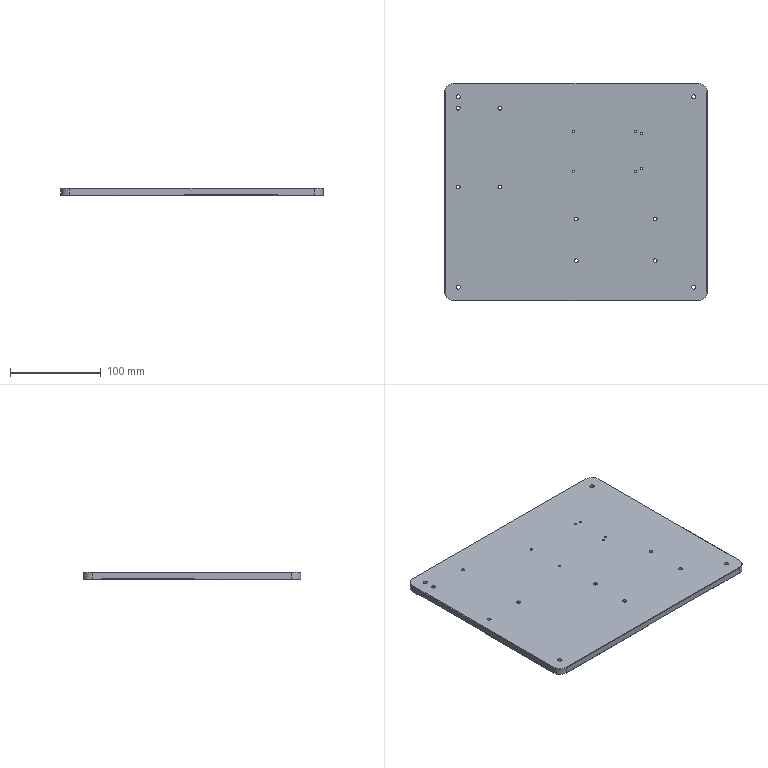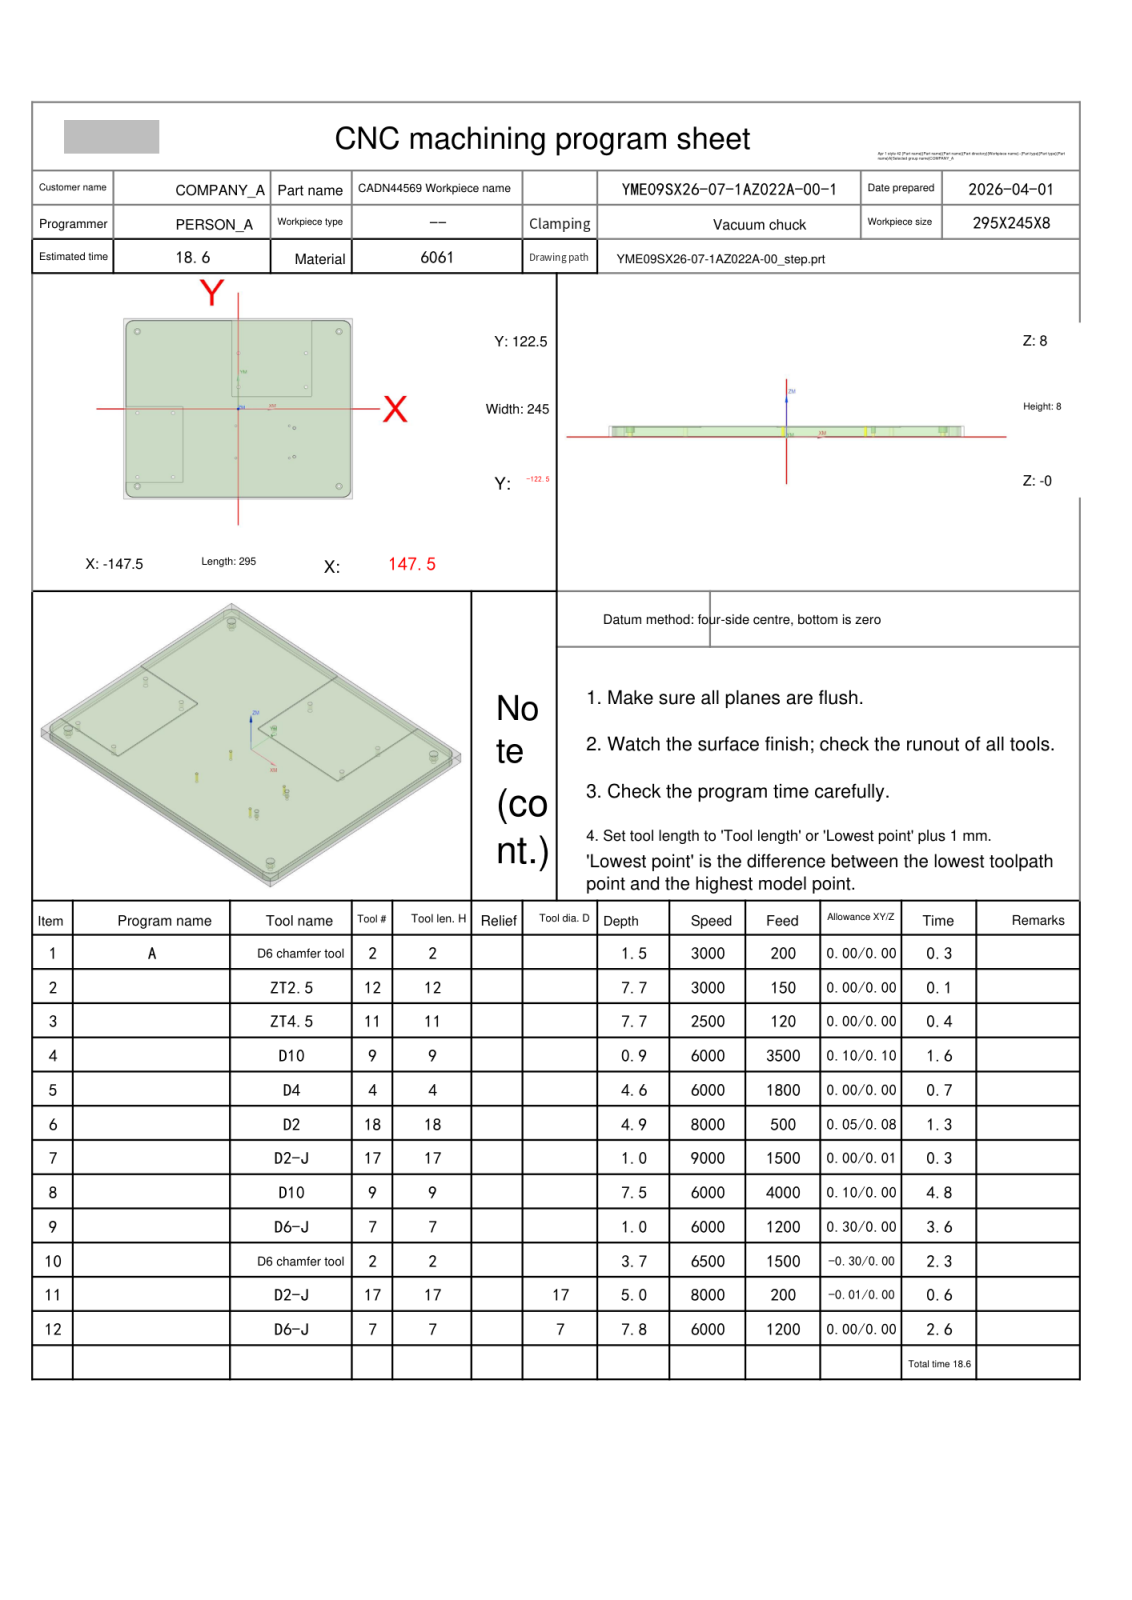NC program | NX | posted by the shop | part box 290 x 240 x 8 mm
Lines 2079 to 2318 of 2318:
N11 T17 M06
(D2-J  D=2. R=0. H=17 ce=-0.01 di=0.00)
G00 G90 G54 X71.195 Y-25.851 M03 S8000
G43 H17 Z28.
M08
Z8.5
G01 Y-25.991 Z8.493 F200.
X71.26 Y-26.261 Z8.478
X71.396 Y-26.503 Z8.464
X71.592 Y-26.699 Z8.449
X71.834 Y-26.835 Z8.434
X72.104 Y-26.9 Z8.42
X72.305 Z8.409
X72.568 Y-26.838 Z8.395
X72.806 Y-26.708 Z8.381
X73. Y-26.521 Z8.367
X73.138 Y-26.288 Z8.353
X73.21 Y-26.027 Z8.339
X73.215 Y-25.79 Z8.326
X73.15 Y-25.52 Z8.312
X73.014 Y-25.278 Z8.297
X72.817 Y-25.081 Z8.282
X72.575 Y-24.945 Z8.268
X72.305 Y-24.88 Z8.253
X72.104 Z8.243
X71.834 Y-24.945 Z8.228
X71.592 Y-25.081 Z8.214
X71.396 Y-25.278 Z8.199
X71.26 Y-25.52 Z8.185
X71.195 Y-25.79 Z8.17
Y-25.991 Z8.159
X71.26 Y-26.261 Z8.145
X71.396 Y-26.503 Z8.13
X71.592 Y-26.699 Z8.116
X71.834 Y-26.835 Z8.101
X72.104 Y-26.9 Z8.087
X72.305 Z8.076
X72.568 Y-26.838 Z8.062
X72.806 Y-26.708 Z8.048
X73. Y-26.521 Z8.034
X73.138 Y-26.288 Z8.019
X73.21 Y-26.027 Z8.005
X73.214 Y-25.927 Z8.
X73.179 Y-25.926
G41 D17
X73.215 Y-25.89
G03 X72.205 Y-24.88 Z7.792 I-1.01 J0.0
X71.195 Y-25.89 Z7.583 I0.0 J-1.01
X72.205 Y-26.9 Z7.375 I1.01 J0.0
X73.215 Y-25.89 Z7.167 I0.0 J1.01
X72.205 Y-24.88 Z6.958 I-1.01 J0.0
X71.195 Y-25.89 Z6.75 I0.0 J-1.01
X72.205 Y-26.9 Z6.542 I1.01 J0.0
X73.215 Y-25.89 Z6.333 I0.0 J1.01
X72.205 Y-24.88 Z6.125 I-1.01 J0.0
X71.195 Y-25.89 Z5.917 I0.0 J-1.01
X72.205 Y-26.9 Z5.708 I1.01 J0.0
X73.215 Y-25.89 Z5.5 I0.0 J1.01
X72.205 Y-24.88 Z5.292 I-1.01 J0.0
X71.195 Y-25.89 Z5.083 I0.0 J-1.01
X72.205 Y-26.9 Z4.875 I1.01 J0.0
X73.215 Y-25.89 Z4.667 I0.0 J1.01
X72.205 Y-24.88 Z4.458 I-1.01 J0.0
X71.195 Y-25.89 Z4.25 I0.0 J-1.01
X72.205 Y-26.9 Z4.042 I1.01 J0.0
X73.215 Y-25.89 Z3.833 I0.0 J1.01
X72.205 Y-24.88 Z3.625 I-1.01 J0.0
X71.195 Y-25.89 Z3.417 I0.0 J-1.01
X72.205 Y-26.9 Z3.208 I1.01 J0.0
X73.215 Y-25.89 Z3. I0.0 J1.01
X72.205 Y-24.88 I-1.01 J0.0
X71.195 Y-25.89 I0.0 J-1.01
X72.205 Y-26.9 I1.01 J0.0
X73.215 Y-25.89 I0.0 J1.01
X73.137 Y-25.501 I-1.01 J0.0
G01 X73.124 Y-25.476
X73.097 Y-25.465
X73.071 Y-25.474
G40 X73.025 Y-25.493
Z4.
G00 Z28.
X72.244 Y-63.88
Z8.5
G01 X72.104 Z8.493
X71.834 Y-63.945 Z8.478
X71.592 Y-64.081 Z8.464
X71.396 Y-64.278 Z8.449
X71.26 Y-64.52 Z8.434
X71.195 Y-64.79 Z8.42
Y-64.991 Z8.409
X71.257 Y-65.254 Z8.395
X71.387 Y-65.491 Z8.381
X71.574 Y-65.686 Z8.367
X71.807 Y-65.824 Z8.353
X72.068 Y-65.896 Z8.339
X72.305 Y-65.9 Z8.326
X72.575 Y-65.835 Z8.312
X72.817 Y-65.699 Z8.297
X73.014 Y-65.503 Z8.282
X73.15 Y-65.261 Z8.268
X73.215 Y-64.991 Z8.253
Y-64.79 Z8.243
X73.15 Y-64.52 Z8.228
X73.014 Y-64.278 Z8.214
X72.817 Y-64.081 Z8.199
X72.575 Y-63.945 Z8.185
X72.305 Y-63.88 Z8.17
X72.104 Z8.159
X71.834 Y-63.945 Z8.145
X71.592 Y-64.081 Z8.13
X71.396 Y-64.278 Z8.116
X71.26 Y-64.52 Z8.101
X71.195 Y-64.79 Z8.087
Y-64.991 Z8.076
X71.257 Y-65.254 Z8.062
X71.387 Y-65.491 Z8.048
X71.574 Y-65.686 Z8.034
X71.807 Y-65.824 Z8.019
X72.068 Y-65.896 Z8.005
X72.168 Y-65.9 Z8.
X72.169 Y-65.865
G41 D17
X72.205 Y-65.9
G03 X73.215 Y-64.89 Z7.792 I0.0 J1.01
X72.205 Y-63.88 Z7.583 I-1.01 J0.0
X71.195 Y-64.89 Z7.375 I0.0 J-1.01
X72.205 Y-65.9 Z7.167 I1.01 J0.0
X73.215 Y-64.89 Z6.958 I0.0 J1.01
X72.205 Y-63.88 Z6.75 I-1.01 J0.0
X71.195 Y-64.89 Z6.542 I0.0 J-1.01
X72.205 Y-65.9 Z6.333 I1.01 J0.0
X73.215 Y-64.89 Z6.125 I0.0 J1.01
X72.205 Y-63.88 Z5.917 I-1.01 J0.0
X71.195 Y-64.89 Z5.708 I0.0 J-1.01
X72.205 Y-65.9 Z5.5 I1.01 J0.0
X73.215 Y-64.89 Z5.292 I0.0 J1.01
X72.205 Y-63.88 Z5.083 I-1.01 J0.0
X71.195 Y-64.89 Z4.875 I0.0 J-1.01
X72.205 Y-65.9 Z4.667 I1.01 J0.0
X73.215 Y-64.89 Z4.458 I0.0 J1.01
X72.205 Y-63.88 Z4.25 I-1.01 J0.0
X71.195 Y-64.89 Z4.042 I0.0 J-1.01
X72.205 Y-65.9 Z3.833 I1.01 J0.0
X73.215 Y-64.89 Z3.625 I0.0 J1.01
X72.205 Y-63.88 Z3.417 I-1.01 J0.0
X71.195 Y-64.89 Z3.208 I0.0 J-1.01
X72.205 Y-65.9 Z3. I1.01 J0.0
X73.215 Y-64.89 I0.0 J1.01
X72.205 Y-63.88 I-1.01 J0.0
X71.195 Y-64.89 I0.0 J-1.01
X72.205 Y-65.9 I1.01 J0.0
X72.594 Y-65.822 I0.0 J1.01
G01 X72.619 Y-65.809
X72.63 Y-65.783
X72.621 Y-65.757
G40 X72.602 Y-65.711
Z4.
G00 Z28.
G91 G28 Z0.0
M05
M09
G91 G28 Z0.0
M01
N12 T07 M06
(D6-J  D=6. R=0. H=07 ce=0.00 di=0.01)
G00 G90 G54 X-4.089 Y123.7 M03 S6000
G43 H07 Z28.
M08
Z7.505
G01 Z7.005 F1200.
G41 D07
X-4.189
G03 X-5.189 Y122.7 I0.0 J-1.
G01 Y19.713
X91.811
Y122.7
G03 X90.811 Y123.7 I-1. J0.0
G01 G40 X90.711
Z7.505
G00 Z28.
G00 G90 X-148.7 Y-95.9 M03 S6000
Z28.
Z7.505
G01 Z7.005 F1200.
G41 D07
Y-96.
G03 X-147.7 Y-97. I1. J0.0
G01 X-74.
Y0.0
X-147.7
G03 X-148.7 Y-1. I0.0 J-1.
G01 G40 Y-1.1
Z7.505
G00 Z28.
G00 G90 X-136.007 Y124.164 M03 S6000
Z28.
Z1.
G01 Z.5 F1000.
G41 D07
X-135.999 Y123.964
G03 X-135. Y123. I.999 J.036
G01 X135.
G02 X148. Y110. I0.0 J-13.
G01 Y-110.
G02 X135. Y-123. I-13. J0.0
G01 X-135.
G02 X-148. Y-110. I0.0 J13.
G01 Y110.
G02 X-135. Y123. I13. J0.0
G01 X-134.5
G03 X-133.5 Y124. I0.0 J1.
G01 G40 Y124.2
Z1.
G00 Z28.
G00 G90 X-136.003 Y124.064 M03 S6000
Z28.
Z.7
G01 Z.2 F1000.
G41 D07
X-135.999 Y123.964
G03 X-135. Y123. I.999 J.036
G01 X135.
G02 X148. Y110. I0.0 J-13.
G01 Y-110.
G02 X135. Y-123. I-13. J0.0
G01 X-135.
G02 X-148. Y-110. I0.0 J13.
G01 Y110.
G02 X-135. Y123. I13. J0.0
G01 X-134.5
G03 X-133.5 Y124. I0.0 J1.
G01 G40 Y124.1
Z.7
G00 Z28.
M05
M09
G91 G28 Z0.0
G91 G28 Y0.0
M30
%